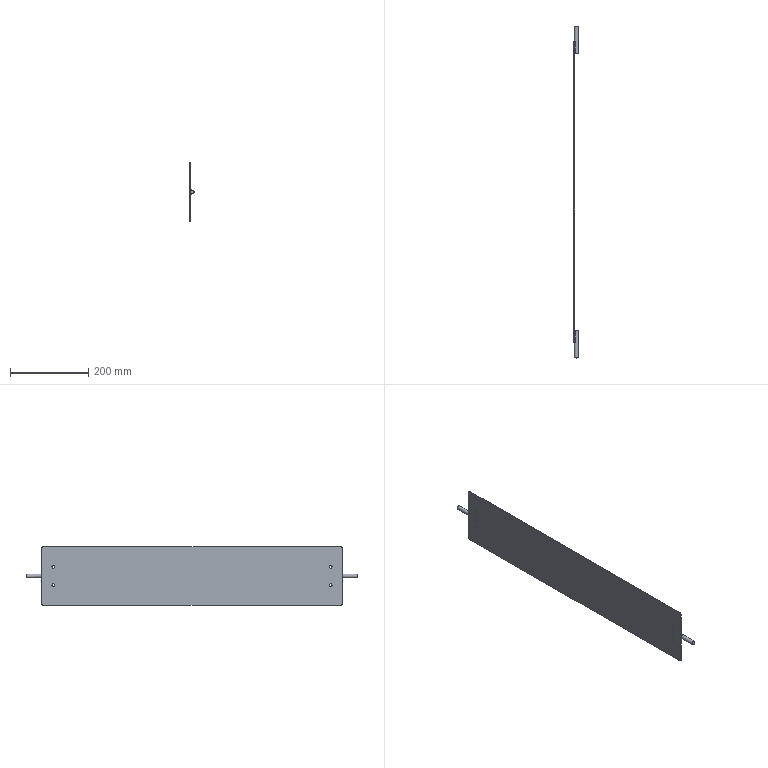Part | NX | features BLEND 3, DATUM_CSYS 3, EXTRUDE 3, SKETCH 2, CPROJ 1 | 1 solid | 24 faces | box 10.5 x 850 x 150 mm | volume 184232 mm3 | cylinder 14 | plane 10 | commonest cylinder face diameters 10 x6 6 x4 7 x4
STEP:
#1=CARTESIAN_POINT('',(1.5,30.,82.937));
#2=VERTEX_POINT('',#1);
#3=CARTESIAN_POINT('',(1.5,30.,67.063));
#4=VERTEX_POINT('',#3);
#5=CARTESIAN_POINT('',(1.5,30.,145.));
#6=DIRECTION('',(0.,0.,-1.));
#7=VECTOR('',#6,1000.);
#8=LINE('',#5,#7);
#9=EDGE_CURVE('',#2,#4,#8,.T.);
#10=ORIENTED_EDGE('',*,*,#9,.T.);
#11=CARTESIAN_POINT('',(1.5,0.,67.063));
#12=VERTEX_POINT('',#11);
#13=CARTESIAN_POINT('',(1.5,5.,67.063));
#14=DIRECTION('',(0.,1.,0.));
#15=VECTOR('',#14,1000.);
#16=LINE('',#13,#15);
#17=EDGE_CURVE('',#4,#12,#16,.F.);
#18=ORIENTED_EDGE('',*,*,#17,.T.);
#19=CARTESIAN_POINT('',(1.5,0.,5.));
#20=VERTEX_POINT('',#19);
#21=CARTESIAN_POINT('',(1.5,0.,5.));
#22=DIRECTION('',(0.,0.,1.));
#23=VECTOR('',#22,1000.);
#24=LINE('',#21,#23);
#25=EDGE_CURVE('',#20,#12,#24,.T.);
#26=ORIENTED_EDGE('',*,*,#25,.F.);
#27=CARTESIAN_POINT('',(1.5,5.,0.));
#28=VERTEX_POINT('',#27);
#29=CARTESIAN_POINT('',(1.5,5.,5.));
#30=DIRECTION('',(-1.,0.,0.));
#31=DIRECTION('',(0.,1.,0.));
#32=AXIS2_PLACEMENT_3D('',#29,#30,#31);
#33=CIRCLE('',#32,5.);
#34=EDGE_CURVE('',#28,#20,#33,.T.);
#35=ORIENTED_EDGE('',*,*,#34,.F.);
#36=CARTESIAN_POINT('',(1.5,765.,0.));
#37=VERTEX_POINT('',#36);
#38=CARTESIAN_POINT('',(1.5,765.,0.));
#39=DIRECTION('',(0.,-1.,0.));
#40=VECTOR('',#39,1000.);
#41=LINE('',#38,#40);
#42=EDGE_CURVE('',#37,#28,#41,.T.);
#43=ORIENTED_EDGE('',*,*,#42,.F.);
#44=CARTESIAN_POINT('',(1.5,770.,5.));
#45=VERTEX_POINT('',#44);
#46=CARTESIAN_POINT('',(1.5,765.,5.));
#47=DIRECTION('',(-1.,0.,0.));
#48=DIRECTION('',(0.,1.,0.));
#49=AXIS2_PLACEMENT_3D('',#46,#47,#48);
#50=CIRCLE('',#49,5.);
#51=EDGE_CURVE('',#45,#37,#50,.T.);
#52=ORIENTED_EDGE('',*,*,#51,.F.);
#53=CARTESIAN_POINT('',(1.5,770.,67.063));
#54=VERTEX_POINT('',#53);
#55=CARTESIAN_POINT('',(1.5,770.,145.));
#56=DIRECTION('',(0.,0.,-1.));
#57=VECTOR('',#56,1000.);
#58=LINE('',#55,#57);
#59=EDGE_CURVE('',#54,#45,#58,.T.);
#60=ORIENTED_EDGE('',*,*,#59,.F.);
#61=CARTESIAN_POINT('',(1.5,740.,67.063));
#62=VERTEX_POINT('',#61);
#63=CARTESIAN_POINT('',(1.5,740.,67.063));
#64=DIRECTION('',(0.,1.,0.));
#65=VECTOR('',#64,1000.);
#66=LINE('',#63,#65);
#67=EDGE_CURVE('',#54,#62,#66,.F.);
#68=ORIENTED_EDGE('',*,*,#67,.T.);
#69=CARTESIAN_POINT('',(1.5,740.,82.937));
#70=VERTEX_POINT('',#69);
#71=CARTESIAN_POINT('',(1.5,740.,145.));
#72=DIRECTION('',(0.,0.,-1.));
#73=VECTOR('',#72,1000.);
#74=LINE('',#71,#73);
#75=EDGE_CURVE('',#70,#62,#74,.T.);
#76=ORIENTED_EDGE('',*,*,#75,.F.);
#77=CARTESIAN_POINT('',(1.5,770.,82.937));
#78=VERTEX_POINT('',#77);
#79=CARTESIAN_POINT('',(1.5,770.,82.937));
#80=DIRECTION('',(0.,1.,0.));
#81=VECTOR('',#80,1000.);
#82=LINE('',#79,#81);
#83=EDGE_CURVE('',#70,#78,#82,.T.);
#84=ORIENTED_EDGE('',*,*,#83,.T.);
#85=CARTESIAN_POINT('',(1.5,770.,145.));
#86=VERTEX_POINT('',#85);
#87=CARTESIAN_POINT('',(1.5,770.,145.));
#88=DIRECTION('',(0.,0.,-1.));
#89=VECTOR('',#88,1000.);
#90=LINE('',#87,#89);
#91=EDGE_CURVE('',#86,#78,#90,.T.);
#92=ORIENTED_EDGE('',*,*,#91,.F.);
#93=CARTESIAN_POINT('',(1.5,765.,150.));
#94=VERTEX_POINT('',#93);
#95=CARTESIAN_POINT('',(1.5,765.,145.));
#96=DIRECTION('',(-1.,0.,0.));
#97=DIRECTION('',(0.,1.,0.));
#98=AXIS2_PLACEMENT_3D('',#95,#96,#97);
#99=CIRCLE('',#98,5.);
#100=EDGE_CURVE('',#94,#86,#99,.T.);
#101=ORIENTED_EDGE('',*,*,#100,.F.);
#102=CARTESIAN_POINT('',(1.5,5.,150.));
#103=VERTEX_POINT('',#102);
#104=CARTESIAN_POINT('',(1.5,5.,150.));
#105=DIRECTION('',(0.,1.,0.));
#106=VECTOR('',#105,1000.);
#107=LINE('',#104,#106);
#108=EDGE_CURVE('',#103,#94,#107,.T.);
#109=ORIENTED_EDGE('',*,*,#108,.F.);
#110=CARTESIAN_POINT('',(1.5,0.,145.));
#111=VERTEX_POINT('',#110);
#112=CARTESIAN_POINT('',(1.5,5.,145.));
#113=DIRECTION('',(-1.,0.,0.));
#114=DIRECTION('',(0.,1.,0.));
#115=AXIS2_PLACEMENT_3D('',#112,#113,#114);
#116=CIRCLE('',#115,5.);
#117=EDGE_CURVE('',#111,#103,#116,.T.);
#118=ORIENTED_EDGE('',*,*,#117,.F.);
#119=CARTESIAN_POINT('',(1.5,0.,82.937));
#120=VERTEX_POINT('',#119);
#121=CARTESIAN_POINT('',(1.5,0.,5.));
#122=DIRECTION('',(0.,0.,1.));
#123=VECTOR('',#122,1000.);
#124=LINE('',#121,#123);
#125=EDGE_CURVE('',#120,#111,#124,.T.);
#126=ORIENTED_EDGE('',*,*,#125,.F.);
#127=CARTESIAN_POINT('',(1.5,5.,82.937));
#128=DIRECTION('',(0.,1.,0.));
#129=VECTOR('',#128,1000.);
#130=LINE('',#127,#129);
#131=EDGE_CURVE('',#120,#2,#130,.T.);
#132=ORIENTED_EDGE('',*,*,#131,.T.);
#133=EDGE_LOOP('',(#10,#18,#26,#35,#43,#52,#60,#68,#76,#84,#92,#101,#109,#118,#126,#132));
#134=FACE_BOUND('',#133,.T.);
#135=CARTESIAN_POINT('',(1.5,33.5,51.5));
#136=VERTEX_POINT('',#135);
#137=CARTESIAN_POINT('',(1.5,30.,51.5));
#138=DIRECTION('',(1.,0.,0.));
#139=DIRECTION('',(0.,1.,0.));
#140=AXIS2_PLACEMENT_3D('',#137,#138,#139);
#141=CIRCLE('',#140,3.5);
#142=EDGE_CURVE('',#136,#136,#141,.T.);
#143=ORIENTED_EDGE('',*,*,#142,.F.);
#144=EDGE_LOOP('',(#143));
#145=FACE_BOUND('',#144,.T.);
#146=CARTESIAN_POINT('',(1.5,33.5,98.5));
#147=VERTEX_POINT('',#146);
#148=CARTESIAN_POINT('',(1.5,30.,98.5));
#149=DIRECTION('',(1.,0.,0.));
#150=DIRECTION('',(0.,1.,0.));
#151=AXIS2_PLACEMENT_3D('',#148,#149,#150);
#152=CIRCLE('',#151,3.5);
#153=EDGE_CURVE('',#147,#147,#152,.T.);
#154=ORIENTED_EDGE('',*,*,#153,.F.);
#155=EDGE_LOOP('',(#154));
#156=FACE_BOUND('',#155,.T.);
#157=CARTESIAN_POINT('',(1.5,743.5,51.5));
#158=VERTEX_POINT('',#157);
#159=CARTESIAN_POINT('',(1.5,740.,51.5));
#160=DIRECTION('',(1.,0.,0.));
#161=DIRECTION('',(0.,1.,0.));
#162=AXIS2_PLACEMENT_3D('',#159,#160,#161);
#163=CIRCLE('',#162,3.5);
#164=EDGE_CURVE('',#158,#158,#163,.T.);
#165=ORIENTED_EDGE('',*,*,#164,.F.);
#166=EDGE_LOOP('',(#165));
#167=FACE_BOUND('',#166,.T.);
#168=CARTESIAN_POINT('',(1.5,743.5,98.5));
#169=VERTEX_POINT('',#168);
#170=CARTESIAN_POINT('',(1.5,740.,98.5));
#171=DIRECTION('',(1.,0.,0.));
#172=DIRECTION('',(0.,1.,0.));
#173=AXIS2_PLACEMENT_3D('',#170,#171,#172);
#174=CIRCLE('',#173,3.5);
#175=EDGE_CURVE('',#169,#169,#174,.T.);
#176=ORIENTED_EDGE('',*,*,#175,.F.);
#177=EDGE_LOOP('',(#176));
#178=FACE_BOUND('',#177,.T.);
#179=CARTESIAN_POINT('',(1.5,5.,145.));
#180=DIRECTION('',(-1.,0.,0.));
#181=DIRECTION('',(0.,0.,1.));
#182=AXIS2_PLACEMENT_3D('',#179,#180,#181);
#183=PLANE('',#182);
#184=ADVANCED_FACE('',(#134,#145,#156,#167,#178),#183,.F.);
#185=CARTESIAN_POINT('',(4.875,0.,79.961));
#186=VERTEX_POINT('',#185);
#187=CARTESIAN_POINT('',(4.875,0.,70.039));
#188=VERTEX_POINT('',#187);
#189=CARTESIAN_POINT('',(5.5,0.,75.));
#190=DIRECTION('',(0.,-1.,0.));
#191=DIRECTION('',(0.,0.,-1.));
#192=AXIS2_PLACEMENT_3D('',#189,#190,#191);
#193=CIRCLE('',#192,5.);
#194=EDGE_CURVE('',#186,#188,#193,.T.);
#195=ORIENTED_EDGE('',*,*,#194,.F.);
#196=CARTESIAN_POINT('',(4.5,0.,82.937));
#197=DIRECTION('',(0.,-1.,0.));
#198=DIRECTION('',(0.,0.,-1.));
#199=AXIS2_PLACEMENT_3D('',#196,#197,#198);
#200=CIRCLE('',#199,3.);
#201=EDGE_CURVE('',#186,#120,#200,.F.);
#202=ORIENTED_EDGE('',*,*,#201,.T.);
#203=ORIENTED_EDGE('',*,*,#125,.T.);
#204=CARTESIAN_POINT('',(0.,0.,145.));
#205=VERTEX_POINT('',#204);
#206=CARTESIAN_POINT('',(1.5,0.,145.));
#207=DIRECTION('',(-1.,0.,0.));
#208=VECTOR('',#207,1000.);
#209=LINE('',#206,#208);
#210=EDGE_CURVE('',#111,#205,#209,.T.);
#211=ORIENTED_EDGE('',*,*,#210,.T.);
#212=CARTESIAN_POINT('',(0.,0.,5.));
#213=VERTEX_POINT('',#212);
#214=CARTESIAN_POINT('',(0.,0.,5.));
#215=DIRECTION('',(0.,0.,1.));
#216=VECTOR('',#215,1000.);
#217=LINE('',#214,#216);
#218=EDGE_CURVE('',#213,#205,#217,.T.);
#219=ORIENTED_EDGE('',*,*,#218,.F.);
#220=CARTESIAN_POINT('',(1.5,0.,5.));
#221=DIRECTION('',(-1.,0.,0.));
#222=VECTOR('',#221,1000.);
#223=LINE('',#220,#222);
#224=EDGE_CURVE('',#20,#213,#223,.T.);
#225=ORIENTED_EDGE('',*,*,#224,.F.);
#226=ORIENTED_EDGE('',*,*,#25,.T.);
#227=CARTESIAN_POINT('',(4.5,0.,67.063));
#228=DIRECTION('',(0.,-1.,0.));
#229=DIRECTION('',(0.,0.,-1.));
#230=AXIS2_PLACEMENT_3D('',#227,#228,#229);
#231=CIRCLE('',#230,3.);
#232=EDGE_CURVE('',#12,#188,#231,.F.);
#233=ORIENTED_EDGE('',*,*,#232,.T.);
#234=EDGE_LOOP('',(#195,#202,#203,#211,#219,#225,#226,#233));
#235=FACE_BOUND('',#234,.T.);
#236=CARTESIAN_POINT('',(1.5,0.,5.));
#237=DIRECTION('',(0.,-1.,0.));
#238=DIRECTION('',(0.,0.,-1.));
#239=AXIS2_PLACEMENT_3D('',#236,#237,#238);
#240=PLANE('',#239);
#241=ADVANCED_FACE('',(#235),#240,.T.);
#242=CARTESIAN_POINT('',(0.,5.,150.));
#243=VERTEX_POINT('',#242);
#244=CARTESIAN_POINT('',(0.,5.,145.));
#245=DIRECTION('',(-1.,0.,0.));
#246=DIRECTION('',(0.,1.,0.));
#247=AXIS2_PLACEMENT_3D('',#244,#245,#246);
#248=CIRCLE('',#247,5.);
#249=EDGE_CURVE('',#205,#243,#248,.T.);
#250=ORIENTED_EDGE('',*,*,#249,.F.);
#251=ORIENTED_EDGE('',*,*,#210,.F.);
#252=ORIENTED_EDGE('',*,*,#117,.T.);
#253=CARTESIAN_POINT('',(1.5,5.,150.));
#254=DIRECTION('',(-1.,0.,0.));
#255=VECTOR('',#254,1000.);
#256=LINE('',#253,#255);
#257=EDGE_CURVE('',#103,#243,#256,.T.);
#258=ORIENTED_EDGE('',*,*,#257,.T.);
#259=EDGE_LOOP('',(#250,#251,#252,#258));
#260=FACE_BOUND('',#259,.T.);
#261=CARTESIAN_POINT('',(1.5,5.,145.));
#262=DIRECTION('',(-1.,0.,0.));
#263=DIRECTION('',(0.,0.,1.));
#264=AXIS2_PLACEMENT_3D('',#261,#262,#263);
#265=CYLINDRICAL_SURFACE('',#264,5.);
#266=ADVANCED_FACE('',(#260),#265,.T.);
#267=CARTESIAN_POINT('',(0.,765.,150.));
#268=VERTEX_POINT('',#267);
#269=CARTESIAN_POINT('',(0.,5.,150.));
#270=DIRECTION('',(0.,1.,0.));
#271=VECTOR('',#270,1000.);
#272=LINE('',#269,#271);
#273=EDGE_CURVE('',#243,#268,#272,.T.);
#274=ORIENTED_EDGE('',*,*,#273,.F.);
#275=ORIENTED_EDGE('',*,*,#257,.F.);
#276=ORIENTED_EDGE('',*,*,#108,.T.);
#277=CARTESIAN_POINT('',(1.5,765.,150.));
#278=DIRECTION('',(-1.,0.,0.));
#279=VECTOR('',#278,1000.);
#280=LINE('',#277,#279);
#281=EDGE_CURVE('',#94,#268,#280,.T.);
#282=ORIENTED_EDGE('',*,*,#281,.T.);
#283=EDGE_LOOP('',(#274,#275,#276,#282));
#284=FACE_BOUND('',#283,.T.);
#285=CARTESIAN_POINT('',(1.5,5.,150.));
#286=DIRECTION('',(0.,0.,1.));
#287=DIRECTION('',(1.,0.,0.));
#288=AXIS2_PLACEMENT_3D('',#285,#286,#287);
#289=PLANE('',#288);
#290=ADVANCED_FACE('',(#284),#289,.T.);
#291=CARTESIAN_POINT('',(0.,770.,145.));
#292=VERTEX_POINT('',#291);
#293=CARTESIAN_POINT('',(0.,765.,145.));
#294=DIRECTION('',(-1.,0.,0.));
#295=DIRECTION('',(0.,1.,0.));
#296=AXIS2_PLACEMENT_3D('',#293,#294,#295);
#297=CIRCLE('',#296,5.);
#298=EDGE_CURVE('',#268,#292,#297,.T.);
#299=ORIENTED_EDGE('',*,*,#298,.F.);
#300=ORIENTED_EDGE('',*,*,#281,.F.);
#301=ORIENTED_EDGE('',*,*,#100,.T.);
#302=CARTESIAN_POINT('',(1.5,770.,145.));
#303=DIRECTION('',(-1.,0.,0.));
#304=VECTOR('',#303,1000.);
#305=LINE('',#302,#304);
#306=EDGE_CURVE('',#86,#292,#305,.T.);
#307=ORIENTED_EDGE('',*,*,#306,.T.);
#308=EDGE_LOOP('',(#299,#300,#301,#307));
#309=FACE_BOUND('',#308,.T.);
#310=CARTESIAN_POINT('',(1.5,765.,145.));
#311=DIRECTION('',(-1.,0.,0.));
#312=DIRECTION('',(0.,0.,1.));
#313=AXIS2_PLACEMENT_3D('',#310,#311,#312);
#314=CYLINDRICAL_SURFACE('',#313,5.);
#315=ADVANCED_FACE('',(#309),#314,.T.);
#316=ORIENTED_EDGE('',*,*,#91,.T.);
#317=CARTESIAN_POINT('',(4.875,770.,79.961));
#318=VERTEX_POINT('',#317);
#319=CARTESIAN_POINT('',(4.5,770.,82.937));
#320=DIRECTION('',(0.,1.,0.));
#321=DIRECTION('',(0.,0.,1.));
#322=AXIS2_PLACEMENT_3D('',#319,#320,#321);
#323=CIRCLE('',#322,3.);
#324=EDGE_CURVE('',#78,#318,#323,.F.);
#325=ORIENTED_EDGE('',*,*,#324,.T.);
#326=CARTESIAN_POINT('',(4.875,770.,70.039));
#327=VERTEX_POINT('',#326);
#328=CARTESIAN_POINT('',(5.5,770.,75.));
#329=DIRECTION('',(0.,1.,0.));
#330=DIRECTION('',(0.,0.,1.));
#331=AXIS2_PLACEMENT_3D('',#328,#329,#330);
#332=CIRCLE('',#331,5.);
#333=EDGE_CURVE('',#318,#327,#332,.F.);
#334=ORIENTED_EDGE('',*,*,#333,.T.);
#335=CARTESIAN_POINT('',(4.5,770.,67.063));
#336=DIRECTION('',(0.,1.,0.));
#337=DIRECTION('',(0.,0.,1.));
#338=AXIS2_PLACEMENT_3D('',#335,#336,#337);
#339=CIRCLE('',#338,3.);
#340=EDGE_CURVE('',#327,#54,#339,.F.);
#341=ORIENTED_EDGE('',*,*,#340,.T.);
#342=ORIENTED_EDGE('',*,*,#59,.T.);
#343=CARTESIAN_POINT('',(0.,770.,5.));
#344=VERTEX_POINT('',#343);
#345=CARTESIAN_POINT('',(1.5,770.,5.));
#346=DIRECTION('',(-1.,0.,0.));
#347=VECTOR('',#346,1000.);
#348=LINE('',#345,#347);
#349=EDGE_CURVE('',#45,#344,#348,.T.);
#350=ORIENTED_EDGE('',*,*,#349,.T.);
#351=CARTESIAN_POINT('',(0.,770.,145.));
#352=DIRECTION('',(0.,0.,-1.));
#353=VECTOR('',#352,1000.);
#354=LINE('',#351,#353);
#355=EDGE_CURVE('',#292,#344,#354,.T.);
#356=ORIENTED_EDGE('',*,*,#355,.F.);
#357=ORIENTED_EDGE('',*,*,#306,.F.);
#358=EDGE_LOOP('',(#316,#325,#334,#341,#342,#350,#356,#357));
#359=FACE_BOUND('',#358,.T.);
#360=CARTESIAN_POINT('',(1.5,770.,145.));
#361=DIRECTION('',(0.,1.,0.));
#362=DIRECTION('',(0.,0.,1.));
#363=AXIS2_PLACEMENT_3D('',#360,#361,#362);
#364=PLANE('',#363);
#365=ADVANCED_FACE('',(#359),#364,.T.);
#366=CARTESIAN_POINT('',(0.,765.,0.));
#367=VERTEX_POINT('',#366);
#368=CARTESIAN_POINT('',(0.,765.,5.));
#369=DIRECTION('',(-1.,0.,0.));
#370=DIRECTION('',(0.,1.,0.));
#371=AXIS2_PLACEMENT_3D('',#368,#369,#370);
#372=CIRCLE('',#371,5.);
#373=EDGE_CURVE('',#344,#367,#372,.T.);
#374=ORIENTED_EDGE('',*,*,#373,.F.);
#375=ORIENTED_EDGE('',*,*,#349,.F.);
#376=ORIENTED_EDGE('',*,*,#51,.T.);
#377=CARTESIAN_POINT('',(1.5,765.,0.));
#378=DIRECTION('',(-1.,0.,0.));
#379=VECTOR('',#378,1000.);
#380=LINE('',#377,#379);
#381=EDGE_CURVE('',#37,#367,#380,.T.);
#382=ORIENTED_EDGE('',*,*,#381,.T.);
#383=EDGE_LOOP('',(#374,#375,#376,#382));
#384=FACE_BOUND('',#383,.T.);
#385=CARTESIAN_POINT('',(1.5,765.,5.));
#386=DIRECTION('',(-1.,0.,0.));
#387=DIRECTION('',(0.,0.,1.));
#388=AXIS2_PLACEMENT_3D('',#385,#386,#387);
#389=CYLINDRICAL_SURFACE('',#388,5.);
#390=ADVANCED_FACE('',(#384),#389,.T.);
#391=CARTESIAN_POINT('',(0.,5.,0.));
#392=VERTEX_POINT('',#391);
#393=CARTESIAN_POINT('',(0.,765.,0.));
#394=DIRECTION('',(0.,-1.,0.));
#395=VECTOR('',#394,1000.);
#396=LINE('',#393,#395);
#397=EDGE_CURVE('',#367,#392,#396,.T.);
#398=ORIENTED_EDGE('',*,*,#397,.F.);
#399=ORIENTED_EDGE('',*,*,#381,.F.);
#400=ORIENTED_EDGE('',*,*,#42,.T.);
#401=CARTESIAN_POINT('',(1.5,5.,0.));
#402=DIRECTION('',(-1.,0.,0.));
#403=VECTOR('',#402,1000.);
#404=LINE('',#401,#403);
#405=EDGE_CURVE('',#28,#392,#404,.T.);
#406=ORIENTED_EDGE('',*,*,#405,.T.);
#407=EDGE_LOOP('',(#398,#399,#400,#406));
#408=FACE_BOUND('',#407,.T.);
#409=CARTESIAN_POINT('',(1.5,765.,0.));
#410=DIRECTION('',(0.,0.,-1.));
#411=DIRECTION('',(0.,1.,0.));
#412=AXIS2_PLACEMENT_3D('',#409,#410,#411);
#413=PLANE('',#412);
#414=ADVANCED_FACE('',(#408),#413,.T.);
#415=ORIENTED_EDGE('',*,*,#153,.T.);
#416=EDGE_LOOP('',(#415));
#417=FACE_BOUND('',#416,.T.);
#418=CARTESIAN_POINT('',(0.,33.5,98.5));
#419=VERTEX_POINT('',#418);
#420=CARTESIAN_POINT('',(0.,30.,98.5));
#421=DIRECTION('',(1.,0.,0.));
#422=DIRECTION('',(0.,1.,0.));
#423=AXIS2_PLACEMENT_3D('',#420,#421,#422);
#424=CIRCLE('',#423,3.5);
#425=EDGE_CURVE('',#419,#419,#424,.T.);
#426=ORIENTED_EDGE('',*,*,#425,.F.);
#427=EDGE_LOOP('',(#426));
#428=FACE_BOUND('',#427,.T.);
#429=CARTESIAN_POINT('',(1.5,30.,98.5));
#430=DIRECTION('',(-1.,0.,0.));
#431=DIRECTION('',(0.,0.,1.));
#432=AXIS2_PLACEMENT_3D('',#429,#430,#431);
#433=CYLINDRICAL_SURFACE('',#432,3.5);
#434=ADVANCED_FACE('',(#417,#428),#433,.F.);
#435=ORIENTED_EDGE('',*,*,#164,.T.);
#436=EDGE_LOOP('',(#435));
#437=FACE_BOUND('',#436,.T.);
#438=CARTESIAN_POINT('',(0.,743.5,51.5));
#439=VERTEX_POINT('',#438);
#440=CARTESIAN_POINT('',(0.,740.,51.5));
#441=DIRECTION('',(1.,0.,0.));
#442=DIRECTION('',(0.,1.,0.));
#443=AXIS2_PLACEMENT_3D('',#440,#441,#442);
#444=CIRCLE('',#443,3.5);
#445=EDGE_CURVE('',#439,#439,#444,.T.);
#446=ORIENTED_EDGE('',*,*,#445,.F.);
#447=EDGE_LOOP('',(#446));
#448=FACE_BOUND('',#447,.T.);
#449=CARTESIAN_POINT('',(1.5,740.,51.5));
#450=DIRECTION('',(-1.,0.,0.));
#451=DIRECTION('',(0.,0.,1.));
#452=AXIS2_PLACEMENT_3D('',#449,#450,#451);
#453=CYLINDRICAL_SURFACE('',#452,3.5);
#454=ADVANCED_FACE('',(#437,#448),#453,.F.);
#455=ORIENTED_EDGE('',*,*,#175,.T.);
#456=EDGE_LOOP('',(#455));
#457=FACE_BOUND('',#456,.T.);
#458=CARTESIAN_POINT('',(0.,743.5,98.5));
#459=VERTEX_POINT('',#458);
#460=CARTESIAN_POINT('',(0.,740.,98.5));
#461=DIRECTION('',(1.,0.,0.));
#462=DIRECTION('',(0.,1.,0.));
#463=AXIS2_PLACEMENT_3D('',#460,#461,#462);
#464=CIRCLE('',#463,3.5);
#465=EDGE_CURVE('',#459,#459,#464,.T.);
#466=ORIENTED_EDGE('',*,*,#465,.F.);
#467=EDGE_LOOP('',(#466));
#468=FACE_BOUND('',#467,.T.);
#469=CARTESIAN_POINT('',(1.5,740.,98.5));
#470=DIRECTION('',(-1.,0.,0.));
#471=DIRECTION('',(0.,0.,1.));
#472=AXIS2_PLACEMENT_3D('',#469,#470,#471);
#473=CYLINDRICAL_SURFACE('',#472,3.5);
#474=ADVANCED_FACE('',(#457,#468),#473,.F.);
#475=CARTESIAN_POINT('',(0.,5.,5.));
#476=DIRECTION('',(-1.,0.,0.));
#477=DIRECTION('',(0.,1.,0.));
#478=AXIS2_PLACEMENT_3D('',#475,#476,#477);
#479=CIRCLE('',#478,5.);
#480=EDGE_CURVE('',#392,#213,#479,.T.);
#481=ORIENTED_EDGE('',*,*,#480,.F.);
#482=ORIENTED_EDGE('',*,*,#405,.F.);
#483=ORIENTED_EDGE('',*,*,#34,.T.);
#484=ORIENTED_EDGE('',*,*,#224,.T.);
#485=EDGE_LOOP('',(#481,#482,#483,#484));
#486=FACE_BOUND('',#485,.T.);
#487=CARTESIAN_POINT('',(1.5,5.,5.));
#488=DIRECTION('',(-1.,0.,0.));
#489=DIRECTION('',(0.,0.,1.));
#490=AXIS2_PLACEMENT_3D('',#487,#488,#489);
#491=CYLINDRICAL_SURFACE('',#490,5.);
#492=ADVANCED_FACE('',(#486),#491,.T.);
#493=ORIENTED_EDGE('',*,*,#142,.T.);
#494=EDGE_LOOP('',(#493));
#495=FACE_BOUND('',#494,.T.);
#496=CARTESIAN_POINT('',(0.,33.5,51.5));
#497=VERTEX_POINT('',#496);
#498=CARTESIAN_POINT('',(0.,30.,51.5));
#499=DIRECTION('',(1.,0.,0.));
#500=DIRECTION('',(0.,1.,0.));
#501=AXIS2_PLACEMENT_3D('',#498,#499,#500);
#502=CIRCLE('',#501,3.5);
#503=EDGE_CURVE('',#497,#497,#502,.T.);
#504=ORIENTED_EDGE('',*,*,#503,.F.);
#505=EDGE_LOOP('',(#504));
#506=FACE_BOUND('',#505,.T.);
#507=CARTESIAN_POINT('',(1.5,30.,51.5));
#508=DIRECTION('',(-1.,0.,0.));
#509=DIRECTION('',(0.,0.,1.));
#510=AXIS2_PLACEMENT_3D('',#507,#508,#509);
#511=CYLINDRICAL_SURFACE('',#510,3.5);
#512=ADVANCED_FACE('',(#495,#506),#511,.F.);
#513=ORIENTED_EDGE('',*,*,#218,.T.);
#514=ORIENTED_EDGE('',*,*,#249,.T.);
#515=ORIENTED_EDGE('',*,*,#273,.T.);
#516=ORIENTED_EDGE('',*,*,#298,.T.);
#517=ORIENTED_EDGE('',*,*,#355,.T.);
#518=ORIENTED_EDGE('',*,*,#373,.T.);
#519=ORIENTED_EDGE('',*,*,#397,.T.);
#520=ORIENTED_EDGE('',*,*,#480,.T.);
#521=EDGE_LOOP('',(#513,#514,#515,#516,#517,#518,#519,#520));
#522=FACE_BOUND('',#521,.T.);
#523=ORIENTED_EDGE('',*,*,#465,.T.);
#524=EDGE_LOOP('',(#523));
#525=FACE_BOUND('',#524,.T.);
#526=ORIENTED_EDGE('',*,*,#445,.T.);
#527=EDGE_LOOP('',(#526));
#528=FACE_BOUND('',#527,.T.);
#529=ORIENTED_EDGE('',*,*,#425,.T.);
#530=EDGE_LOOP('',(#529));
#531=FACE_BOUND('',#530,.T.);
#532=ORIENTED_EDGE('',*,*,#503,.T.);
#533=EDGE_LOOP('',(#532));
#534=FACE_BOUND('',#533,.T.);
#535=CARTESIAN_POINT('',(0.,5.,145.));
#536=DIRECTION('',(-1.,0.,0.));
#537=DIRECTION('',(0.,0.,1.));
#538=AXIS2_PLACEMENT_3D('',#535,#536,#537);
#539=PLANE('',#538);
#540=ADVANCED_FACE('',(#522,#525,#528,#531,#534),#539,.T.);
#541=CARTESIAN_POINT('',(5.5,810.,80.));
#542=VERTEX_POINT('',#541);
#543=CARTESIAN_POINT('',(5.5,810.,75.));
#544=DIRECTION('',(0.,1.,0.));
#545=DIRECTION('',(0.,0.,1.));
#546=AXIS2_PLACEMENT_3D('',#543,#544,#545);
#547=CIRCLE('',#546,5.);
#548=EDGE_CURVE('',#542,#542,#547,.T.);
#549=ORIENTED_EDGE('',*,*,#548,.F.);
#550=EDGE_LOOP('',(#549));
#551=FACE_BOUND('',#550,.T.);
#552=ORIENTED_EDGE('',*,*,#333,.F.);
#553=CARTESIAN_POINT('',(4.875,740.,79.961));
#554=VERTEX_POINT('',#553);
#555=CARTESIAN_POINT('',(4.875,810.,79.961));
#556=DIRECTION('',(0.,-1.,0.));
#557=VECTOR('',#556,1000.);
#558=LINE('',#555,#557);
#559=EDGE_CURVE('',#318,#554,#558,.T.);
#560=ORIENTED_EDGE('',*,*,#559,.T.);
#561=CARTESIAN_POINT('',(4.875,740.,70.039));
#562=VERTEX_POINT('',#561);
#563=CARTESIAN_POINT('',(5.5,740.,75.));
#564=DIRECTION('',(0.,1.,0.));
#565=DIRECTION('',(0.,0.,1.));
#566=AXIS2_PLACEMENT_3D('',#563,#564,#565);
#567=CIRCLE('',#566,5.);
#568=EDGE_CURVE('',#554,#562,#567,.T.);
#569=ORIENTED_EDGE('',*,*,#568,.T.);
#570=CARTESIAN_POINT('',(4.875,810.,70.039));
#571=DIRECTION('',(0.,-1.,0.));
#572=VECTOR('',#571,1000.);
#573=LINE('',#570,#572);
#574=EDGE_CURVE('',#562,#327,#573,.F.);
#575=ORIENTED_EDGE('',*,*,#574,.T.);
#576=EDGE_LOOP('',(#552,#560,#569,#575));
#577=FACE_BOUND('',#576,.T.);
#578=CARTESIAN_POINT('',(5.5,810.,75.));
#579=DIRECTION('',(0.,-1.,0.));
#580=DIRECTION('',(0.,0.,-1.));
#581=AXIS2_PLACEMENT_3D('',#578,#579,#580);
#582=CYLINDRICAL_SURFACE('',#581,5.);
#583=ADVANCED_FACE('',(#551,#577),#582,.T.);
#584=ORIENTED_EDGE('',*,*,#568,.F.);
#585=CARTESIAN_POINT('',(4.5,740.,82.937));
#586=DIRECTION('',(0.,1.,0.));
#587=DIRECTION('',(0.,0.,1.));
#588=AXIS2_PLACEMENT_3D('',#585,#586,#587);
#589=CIRCLE('',#588,3.);
#590=EDGE_CURVE('',#554,#70,#589,.T.);
#591=ORIENTED_EDGE('',*,*,#590,.T.);
#592=ORIENTED_EDGE('',*,*,#75,.T.);
#593=CARTESIAN_POINT('',(4.5,740.,67.063));
#594=DIRECTION('',(0.,1.,0.));
#595=DIRECTION('',(0.,0.,1.));
#596=AXIS2_PLACEMENT_3D('',#593,#594,#595);
#597=CIRCLE('',#596,3.);
#598=EDGE_CURVE('',#62,#562,#597,.T.);
#599=ORIENTED_EDGE('',*,*,#598,.T.);
#600=EDGE_LOOP('',(#584,#591,#592,#599));
#601=FACE_BOUND('',#600,.T.);
#602=CARTESIAN_POINT('',(5.5,740.,75.));
#603=DIRECTION('',(0.,1.,0.));
#604=DIRECTION('',(0.,0.,1.));
#605=AXIS2_PLACEMENT_3D('',#602,#603,#604);
#606=PLANE('',#605);
#607=ADVANCED_FACE('',(#601),#606,.F.);
#608=ORIENTED_EDGE('',*,*,#548,.T.);
#609=EDGE_LOOP('',(#608));
#610=FACE_BOUND('',#609,.T.);
#611=CARTESIAN_POINT('',(5.5,810.,75.));
#612=DIRECTION('',(0.,1.,0.));
#613=DIRECTION('',(0.,0.,1.));
#614=AXIS2_PLACEMENT_3D('',#611,#612,#613);
#615=PLANE('',#614);
#616=ADVANCED_FACE('',(#610),#615,.T.);
#617=ORIENTED_EDGE('',*,*,#598,.F.);
#618=ORIENTED_EDGE('',*,*,#67,.F.);
#619=ORIENTED_EDGE('',*,*,#340,.F.);
#620=ORIENTED_EDGE('',*,*,#574,.F.);
#621=EDGE_LOOP('',(#617,#618,#619,#620));
#622=FACE_BOUND('',#621,.T.);
#623=CARTESIAN_POINT('',(4.5,810.,67.063));
#624=DIRECTION('',(0.,-1.,0.));
#625=DIRECTION('',(0.,0.,-1.));
#626=AXIS2_PLACEMENT_3D('',#623,#624,#625);
#627=CYLINDRICAL_SURFACE('',#626,3.);
#628=ADVANCED_FACE('',(#622),#627,.F.);
#629=ORIENTED_EDGE('',*,*,#324,.F.);
#630=ORIENTED_EDGE('',*,*,#83,.F.);
#631=ORIENTED_EDGE('',*,*,#590,.F.);
#632=ORIENTED_EDGE('',*,*,#559,.F.);
#633=EDGE_LOOP('',(#629,#630,#631,#632));
#634=FACE_BOUND('',#633,.T.);
#635=CARTESIAN_POINT('',(4.5,810.,82.937));
#636=DIRECTION('',(0.,-1.,0.));
#637=DIRECTION('',(0.,0.,-1.));
#638=AXIS2_PLACEMENT_3D('',#635,#636,#637);
#639=CYLINDRICAL_SURFACE('',#638,3.);
#640=ADVANCED_FACE('',(#634),#639,.F.);
#641=ORIENTED_EDGE('',*,*,#9,.F.);
#642=CARTESIAN_POINT('',(4.875,30.,79.961));
#643=VERTEX_POINT('',#642);
#644=CARTESIAN_POINT('',(4.5,30.,82.937));
#645=DIRECTION('',(0.,1.,0.));
#646=DIRECTION('',(0.,0.,1.));
#647=AXIS2_PLACEMENT_3D('',#644,#645,#646);
#648=CIRCLE('',#647,3.);
#649=EDGE_CURVE('',#2,#643,#648,.F.);
#650=ORIENTED_EDGE('',*,*,#649,.T.);
#651=CARTESIAN_POINT('',(4.875,30.,70.039));
#652=VERTEX_POINT('',#651);
#653=CARTESIAN_POINT('',(5.5,30.,75.));
#654=DIRECTION('',(0.,1.,0.));
#655=DIRECTION('',(0.,0.,1.));
#656=AXIS2_PLACEMENT_3D('',#653,#654,#655);
#657=CIRCLE('',#656,5.);
#658=EDGE_CURVE('',#643,#652,#657,.T.);
#659=ORIENTED_EDGE('',*,*,#658,.T.);
#660=CARTESIAN_POINT('',(4.5,30.,67.063));
#661=DIRECTION('',(0.,1.,0.));
#662=DIRECTION('',(0.,0.,1.));
#663=AXIS2_PLACEMENT_3D('',#660,#661,#662);
#664=CIRCLE('',#663,3.);
#665=EDGE_CURVE('',#652,#4,#664,.F.);
#666=ORIENTED_EDGE('',*,*,#665,.T.);
#667=EDGE_LOOP('',(#641,#650,#659,#666));
#668=FACE_BOUND('',#667,.T.);
#669=CARTESIAN_POINT('',(5.5,30.,75.));
#670=DIRECTION('',(0.,1.,0.));
#671=DIRECTION('',(0.,0.,1.));
#672=AXIS2_PLACEMENT_3D('',#669,#670,#671);
#673=PLANE('',#672);
#674=ADVANCED_FACE('',(#668),#673,.T.);
#675=CARTESIAN_POINT('',(5.5,-40.,80.));
#676=VERTEX_POINT('',#675);
#677=CARTESIAN_POINT('',(5.5,-40.,75.));
#678=DIRECTION('',(0.,1.,0.));
#679=DIRECTION('',(0.,0.,1.));
#680=AXIS2_PLACEMENT_3D('',#677,#678,#679);
#681=CIRCLE('',#680,5.);
#682=EDGE_CURVE('',#676,#676,#681,.T.);
#683=ORIENTED_EDGE('',*,*,#682,.T.);
#684=EDGE_LOOP('',(#683));
#685=FACE_BOUND('',#684,.T.);
#686=ORIENTED_EDGE('',*,*,#194,.T.);
#687=CARTESIAN_POINT('',(4.875,-40.,70.039));
#688=DIRECTION('',(0.,1.,0.));
#689=VECTOR('',#688,1000.);
#690=LINE('',#687,#689);
#691=EDGE_CURVE('',#188,#652,#690,.T.);
#692=ORIENTED_EDGE('',*,*,#691,.T.);
#693=ORIENTED_EDGE('',*,*,#658,.F.);
#694=CARTESIAN_POINT('',(4.875,-40.,79.961));
#695=DIRECTION('',(0.,1.,0.));
#696=VECTOR('',#695,1000.);
#697=LINE('',#694,#696);
#698=EDGE_CURVE('',#643,#186,#697,.F.);
#699=ORIENTED_EDGE('',*,*,#698,.T.);
#700=EDGE_LOOP('',(#686,#692,#693,#699));
#701=FACE_BOUND('',#700,.T.);
#702=CARTESIAN_POINT('',(5.5,-40.,75.));
#703=DIRECTION('',(0.,1.,0.));
#704=DIRECTION('',(0.,0.,1.));
#705=AXIS2_PLACEMENT_3D('',#702,#703,#704);
#706=CYLINDRICAL_SURFACE('',#705,5.);
#707=ADVANCED_FACE('',(#685,#701),#706,.T.);
#708=ORIENTED_EDGE('',*,*,#682,.F.);
#709=EDGE_LOOP('',(#708));
#710=FACE_BOUND('',#709,.T.);
#711=CARTESIAN_POINT('',(5.5,-40.,75.));
#712=DIRECTION('',(0.,1.,0.));
#713=DIRECTION('',(0.,0.,1.));
#714=AXIS2_PLACEMENT_3D('',#711,#712,#713);
#715=PLANE('',#714);
#716=ADVANCED_FACE('',(#710),#715,.F.);
#717=ORIENTED_EDGE('',*,*,#665,.F.);
#718=ORIENTED_EDGE('',*,*,#691,.F.);
#719=ORIENTED_EDGE('',*,*,#232,.F.);
#720=ORIENTED_EDGE('',*,*,#17,.F.);
#721=EDGE_LOOP('',(#717,#718,#719,#720));
#722=FACE_BOUND('',#721,.T.);
#723=CARTESIAN_POINT('',(4.5,-40.,67.063));
#724=DIRECTION('',(0.,1.,0.));
#725=DIRECTION('',(0.,0.,1.));
#726=AXIS2_PLACEMENT_3D('',#723,#724,#725);
#727=CYLINDRICAL_SURFACE('',#726,3.);
#728=ADVANCED_FACE('',(#722),#727,.F.);
#729=ORIENTED_EDGE('',*,*,#201,.F.);
#730=ORIENTED_EDGE('',*,*,#698,.F.);
#731=ORIENTED_EDGE('',*,*,#649,.F.);
#732=ORIENTED_EDGE('',*,*,#131,.F.);
#733=EDGE_LOOP('',(#729,#730,#731,#732));
#734=FACE_BOUND('',#733,.T.);
#735=CARTESIAN_POINT('',(4.5,-40.,82.937));
#736=DIRECTION('',(0.,1.,0.));
#737=DIRECTION('',(0.,0.,1.));
#738=AXIS2_PLACEMENT_3D('',#735,#736,#737);
#739=CYLINDRICAL_SURFACE('',#738,3.);
#740=ADVANCED_FACE('',(#734),#739,.F.);
#741=CLOSED_SHELL('',(#184,#241,#266,#290,#315,#365,#390,#414,#434,#454,#474,#492,#512,#540,#583,#607,#616,#628,#640,#674,#707,#716,#728,#740));
#742=MANIFOLD_SOLID_BREP('',#741);
#743=(LENGTH_UNIT()NAMED_UNIT(*)SI_UNIT(.MILLI.,.METRE.));
#744=UNCERTAINTY_MEASURE_WITH_UNIT(LENGTH_MEASURE(0.00001),#743,'','');
#745=(NAMED_UNIT(*)PLANE_ANGLE_UNIT()SI_UNIT($,.RADIAN.));
#746=(NAMED_UNIT(*)SI_UNIT($,.STERADIAN.)SOLID_ANGLE_UNIT());
#747=(GEOMETRIC_REPRESENTATION_CONTEXT(3)GLOBAL_UNCERTAINTY_ASSIGNED_CONTEXT((#744))GLOBAL_UNIT_ASSIGNED_CONTEXT((#743,#745,#746))REPRESENTATION_CONTEXT('',''));
#748=ADVANCED_BREP_SHAPE_REPRESENTATION('',(#742),#747);